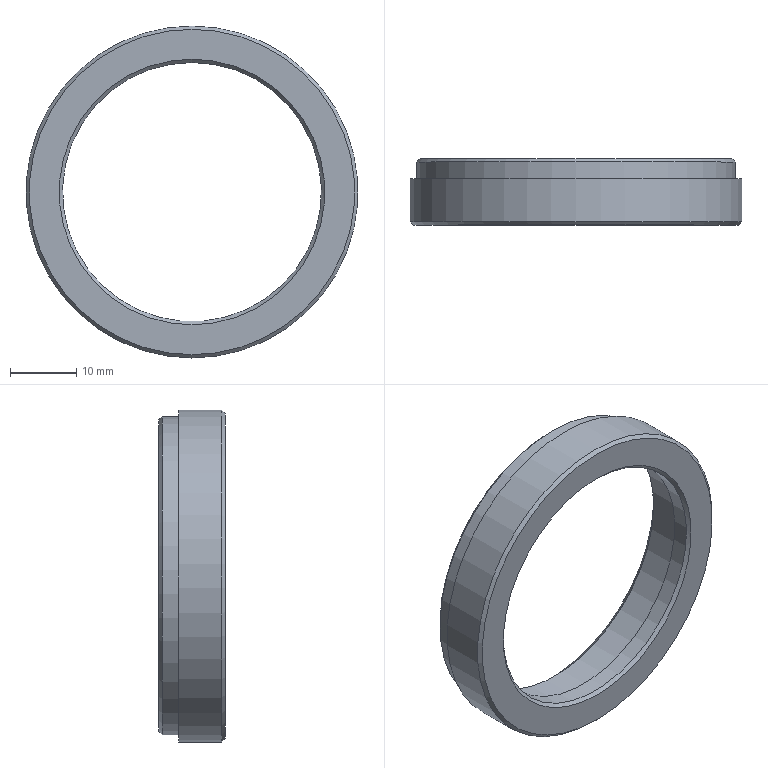Part | STEP file | JBJ-P-1018-01 | 1 solid | 12 faces | box 50 x 10 x 50 mm | volume 5771 mm3 | plane 4 | cylinder 4 | cone 4 | commonest cylinder face diameters 39 x1 42 x1 48 x1 50 x1
STEP:
#1=CARTESIAN_POINT('',(0.,10.,23.5));
#2=VERTEX_POINT('',#1);
#3=CARTESIAN_POINT('',(0.,10.,0.));
#4=DIRECTION('',(0.,1.,0.));
#5=DIRECTION('',(0.,0.,1.));
#6=AXIS2_PLACEMENT_3D('',#3,#4,#5);
#7=CIRCLE('',#6,23.5);
#8=EDGE_CURVE('',#2,#2,#7,.T.);
#9=ORIENTED_EDGE('',*,*,#8,.T.);
#10=EDGE_LOOP('',(#9));
#11=FACE_OUTER_BOUND('',#10,.T.);
#12=CARTESIAN_POINT('',(0.,10.,22.));
#13=VERTEX_POINT('',#12);
#14=CARTESIAN_POINT('',(0.,10.,0.));
#15=DIRECTION('',(0.,-1.,0.));
#16=DIRECTION('',(0.,0.,1.));
#17=AXIS2_PLACEMENT_3D('',#14,#15,#16);
#18=CIRCLE('',#17,22.);
#19=EDGE_CURVE('',#13,#13,#18,.T.);
#20=ORIENTED_EDGE('',*,*,#19,.T.);
#21=EDGE_LOOP('',(#20));
#22=FACE_BOUND('',#21,.T.);
#23=CARTESIAN_POINT('',(0.,10.,0.));
#24=DIRECTION('',(0.,1.,0.));
#25=DIRECTION('',(0.,0.,1.));
#26=AXIS2_PLACEMENT_3D('',#23,#24,#25);
#27=PLANE('',#26);
#28=ADVANCED_FACE('',(#11,#22),#27,.T.);
#29=CARTESIAN_POINT('',(0.,0.5,25.));
#30=VERTEX_POINT('',#29);
#31=CARTESIAN_POINT('',(0.,0.5,0.));
#32=DIRECTION('',(0.,1.,0.));
#33=DIRECTION('',(0.,0.,1.));
#34=AXIS2_PLACEMENT_3D('',#31,#32,#33);
#35=CIRCLE('',#34,25.);
#36=EDGE_CURVE('',#30,#30,#35,.T.);
#37=ORIENTED_EDGE('',*,*,#36,.T.);
#38=EDGE_LOOP('',(#37));
#39=FACE_OUTER_BOUND('',#38,.T.);
#40=CARTESIAN_POINT('',(0.,7.,25.));
#41=VERTEX_POINT('',#40);
#42=CARTESIAN_POINT('',(0.,7.,0.));
#43=DIRECTION('',(0.,1.,0.));
#44=DIRECTION('',(0.,0.,1.));
#45=AXIS2_PLACEMENT_3D('',#42,#43,#44);
#46=CIRCLE('',#45,25.);
#47=EDGE_CURVE('',#41,#41,#46,.T.);
#48=ORIENTED_EDGE('',*,*,#47,.F.);
#49=EDGE_LOOP('',(#48));
#50=FACE_OUTER_BOUND('',#49,.T.);
#51=CARTESIAN_POINT('',(0.,10.,0.));
#52=DIRECTION('',(0.,-1.,0.));
#53=DIRECTION('',(0.,0.,-1.));
#54=AXIS2_PLACEMENT_3D('',#51,#52,#53);
#55=CYLINDRICAL_SURFACE('',#54,25.);
#56=ADVANCED_FACE('',(#39,#50),#55,.T.);
#57=CARTESIAN_POINT('',(0.,0.5,19.5));
#58=VERTEX_POINT('',#57);
#59=CARTESIAN_POINT('',(0.,0.5,0.));
#60=DIRECTION('',(0.,-1.,0.));
#61=DIRECTION('',(0.,0.,1.));
#62=AXIS2_PLACEMENT_3D('',#59,#60,#61);
#63=CIRCLE('',#62,19.5);
#64=EDGE_CURVE('',#58,#58,#63,.T.);
#65=ORIENTED_EDGE('',*,*,#64,.T.);
#66=EDGE_LOOP('',(#65));
#67=FACE_OUTER_BOUND('',#66,.T.);
#68=CARTESIAN_POINT('',(0.,3.,19.5));
#69=VERTEX_POINT('',#68);
#70=CARTESIAN_POINT('',(0.,3.,0.));
#71=DIRECTION('',(0.,1.,0.));
#72=DIRECTION('',(0.,0.,1.));
#73=AXIS2_PLACEMENT_3D('',#70,#71,#72);
#74=CIRCLE('',#73,19.5);
#75=EDGE_CURVE('',#69,#69,#74,.T.);
#76=ORIENTED_EDGE('',*,*,#75,.T.);
#77=EDGE_LOOP('',(#76));
#78=FACE_OUTER_BOUND('',#77,.T.);
#79=CARTESIAN_POINT('',(0.,10.,0.));
#80=DIRECTION('',(0.,-1.,0.));
#81=DIRECTION('',(0.,0.,-1.));
#82=AXIS2_PLACEMENT_3D('',#79,#80,#81);
#83=CYLINDRICAL_SURFACE('',#82,19.5);
#84=ADVANCED_FACE('',(#67,#78),#83,.F.);
#85=CARTESIAN_POINT('',(0.,0.,20.));
#86=VERTEX_POINT('',#85);
#87=CARTESIAN_POINT('',(0.,0.,0.));
#88=DIRECTION('',(0.,1.,0.));
#89=DIRECTION('',(0.,0.,1.));
#90=AXIS2_PLACEMENT_3D('',#87,#88,#89);
#91=CIRCLE('',#90,20.);
#92=EDGE_CURVE('',#86,#86,#91,.T.);
#93=ORIENTED_EDGE('',*,*,#92,.T.);
#94=EDGE_LOOP('',(#93));
#95=FACE_BOUND('',#94,.T.);
#96=CARTESIAN_POINT('',(0.,0.,24.5));
#97=VERTEX_POINT('',#96);
#98=CARTESIAN_POINT('',(0.,0.,0.));
#99=DIRECTION('',(0.,-1.,0.));
#100=DIRECTION('',(0.,0.,1.));
#101=AXIS2_PLACEMENT_3D('',#98,#99,#100);
#102=CIRCLE('',#101,24.5);
#103=EDGE_CURVE('',#97,#97,#102,.T.);
#104=ORIENTED_EDGE('',*,*,#103,.T.);
#105=EDGE_LOOP('',(#104));
#106=FACE_OUTER_BOUND('',#105,.T.);
#107=CARTESIAN_POINT('',(0.,0.,0.));
#108=DIRECTION('',(0.,1.,0.));
#109=DIRECTION('',(0.,0.,1.));
#110=AXIS2_PLACEMENT_3D('',#107,#108,#109);
#111=PLANE('',#110);
#112=ADVANCED_FACE('',(#95,#106),#111,.F.);
#113=CARTESIAN_POINT('',(0.,9.,21.));
#114=VERTEX_POINT('',#113);
#115=CARTESIAN_POINT('',(0.,9.,0.));
#116=DIRECTION('',(0.,1.,0.));
#117=DIRECTION('',(0.,0.,1.));
#118=AXIS2_PLACEMENT_3D('',#115,#116,#117);
#119=CIRCLE('',#118,21.);
#120=EDGE_CURVE('',#114,#114,#119,.T.);
#121=ORIENTED_EDGE('',*,*,#120,.T.);
#122=EDGE_LOOP('',(#121));
#123=FACE_OUTER_BOUND('',#122,.T.);
#124=CARTESIAN_POINT('',(0.,3.,21.));
#125=VERTEX_POINT('',#124);
#126=CARTESIAN_POINT('',(0.,3.,0.));
#127=DIRECTION('',(0.,1.,0.));
#128=DIRECTION('',(0.,0.,1.));
#129=AXIS2_PLACEMENT_3D('',#126,#127,#128);
#130=CIRCLE('',#129,21.);
#131=EDGE_CURVE('',#125,#125,#130,.T.);
#132=ORIENTED_EDGE('',*,*,#131,.F.);
#133=EDGE_LOOP('',(#132));
#134=FACE_OUTER_BOUND('',#133,.T.);
#135=CARTESIAN_POINT('',(0.,3.,0.));
#136=DIRECTION('',(0.,1.,0.));
#137=DIRECTION('',(0.,0.,1.));
#138=AXIS2_PLACEMENT_3D('',#135,#136,#137);
#139=CYLINDRICAL_SURFACE('',#138,21.);
#140=ADVANCED_FACE('',(#123,#134),#139,.F.);
#141=ORIENTED_EDGE('',*,*,#75,.F.);
#142=EDGE_LOOP('',(#141));
#143=FACE_BOUND('',#142,.T.);
#144=ORIENTED_EDGE('',*,*,#131,.T.);
#145=EDGE_LOOP('',(#144));
#146=FACE_OUTER_BOUND('',#145,.T.);
#147=CARTESIAN_POINT('',(0.,3.,0.));
#148=DIRECTION('',(0.,1.,0.));
#149=DIRECTION('',(0.,0.,1.));
#150=AXIS2_PLACEMENT_3D('',#147,#148,#149);
#151=PLANE('',#150);
#152=ADVANCED_FACE('',(#143,#146),#151,.T.);
#153=ORIENTED_EDGE('',*,*,#19,.F.);
#154=EDGE_LOOP('',(#153));
#155=FACE_OUTER_BOUND('',#154,.T.);
#156=ORIENTED_EDGE('',*,*,#120,.F.);
#157=EDGE_LOOP('',(#156));
#158=FACE_BOUND('',#157,.T.);
#159=CARTESIAN_POINT('',(0.,9.,0.));
#160=DIRECTION('',(0.,1.,0.));
#161=DIRECTION('',(0.,0.,1.));
#162=AXIS2_PLACEMENT_3D('',#159,#160,#161);
#163=CONICAL_SURFACE('',#162,21.,0.7854);
#164=ADVANCED_FACE('',(#155,#158),#163,.F.);
#165=CARTESIAN_POINT('',(0.,7.,24.));
#166=VERTEX_POINT('',#165);
#167=CARTESIAN_POINT('',(0.,7.,0.));
#168=DIRECTION('',(0.,1.,0.));
#169=DIRECTION('',(0.,0.,1.));
#170=AXIS2_PLACEMENT_3D('',#167,#168,#169);
#171=CIRCLE('',#170,24.);
#172=EDGE_CURVE('',#166,#166,#171,.T.);
#173=ORIENTED_EDGE('',*,*,#172,.F.);
#174=EDGE_LOOP('',(#173));
#175=FACE_BOUND('',#174,.T.);
#176=ORIENTED_EDGE('',*,*,#47,.T.);
#177=EDGE_LOOP('',(#176));
#178=FACE_OUTER_BOUND('',#177,.T.);
#179=CARTESIAN_POINT('',(0.,7.,0.));
#180=DIRECTION('',(0.,1.,0.));
#181=DIRECTION('',(0.,0.,1.));
#182=AXIS2_PLACEMENT_3D('',#179,#180,#181);
#183=PLANE('',#182);
#184=ADVANCED_FACE('',(#175,#178),#183,.T.);
#185=CARTESIAN_POINT('',(0.,9.5,24.));
#186=VERTEX_POINT('',#185);
#187=CARTESIAN_POINT('',(0.,9.5,0.));
#188=DIRECTION('',(0.,-1.,0.));
#189=DIRECTION('',(0.,0.,1.));
#190=AXIS2_PLACEMENT_3D('',#187,#188,#189);
#191=CIRCLE('',#190,24.);
#192=EDGE_CURVE('',#186,#186,#191,.T.);
#193=ORIENTED_EDGE('',*,*,#192,.T.);
#194=EDGE_LOOP('',(#193));
#195=FACE_OUTER_BOUND('',#194,.T.);
#196=ORIENTED_EDGE('',*,*,#172,.T.);
#197=EDGE_LOOP('',(#196));
#198=FACE_OUTER_BOUND('',#197,.T.);
#199=CARTESIAN_POINT('',(0.,7.,0.));
#200=DIRECTION('',(0.,1.,0.));
#201=DIRECTION('',(0.,0.,1.));
#202=AXIS2_PLACEMENT_3D('',#199,#200,#201);
#203=CYLINDRICAL_SURFACE('',#202,24.);
#204=ADVANCED_FACE('',(#195,#198),#203,.T.);
#205=ORIENTED_EDGE('',*,*,#64,.F.);
#206=EDGE_LOOP('',(#205));
#207=FACE_BOUND('',#206,.T.);
#208=ORIENTED_EDGE('',*,*,#92,.F.);
#209=EDGE_LOOP('',(#208));
#210=FACE_OUTER_BOUND('',#209,.T.);
#211=CARTESIAN_POINT('',(0.,0.,0.));
#212=DIRECTION('',(0.,-1.,0.));
#213=DIRECTION('',(0.,0.,-1.));
#214=AXIS2_PLACEMENT_3D('',#211,#212,#213);
#215=CONICAL_SURFACE('',#214,20.,0.7854);
#216=ADVANCED_FACE('',(#207,#210),#215,.F.);
#217=ORIENTED_EDGE('',*,*,#103,.F.);
#218=EDGE_LOOP('',(#217));
#219=FACE_BOUND('',#218,.T.);
#220=ORIENTED_EDGE('',*,*,#36,.F.);
#221=EDGE_LOOP('',(#220));
#222=FACE_OUTER_BOUND('',#221,.T.);
#223=CARTESIAN_POINT('',(0.,0.5,0.));
#224=DIRECTION('',(0.,1.,0.));
#225=DIRECTION('',(0.,0.,1.));
#226=AXIS2_PLACEMENT_3D('',#223,#224,#225);
#227=CONICAL_SURFACE('',#226,25.,0.7854);
#228=ADVANCED_FACE('',(#219,#222),#227,.T.);
#229=ORIENTED_EDGE('',*,*,#192,.F.);
#230=EDGE_LOOP('',(#229));
#231=FACE_OUTER_BOUND('',#230,.T.);
#232=ORIENTED_EDGE('',*,*,#8,.F.);
#233=EDGE_LOOP('',(#232));
#234=FACE_BOUND('',#233,.T.);
#235=CARTESIAN_POINT('',(0.,10.,0.));
#236=DIRECTION('',(0.,-1.,0.));
#237=DIRECTION('',(0.,0.,-1.));
#238=AXIS2_PLACEMENT_3D('',#235,#236,#237);
#239=CONICAL_SURFACE('',#238,23.5,0.7854);
#240=ADVANCED_FACE('',(#231,#234),#239,.T.);
#241=CLOSED_SHELL('',(#28,#56,#84,#112,#140,#152,#164,#184,#204,#216,#228,#240));
#242=MANIFOLD_SOLID_BREP('',#241);
#243=CARTESIAN_POINT('',(0.,0.,0.));
#244=DIRECTION('',(0.,0.,1.));
#245=DIRECTION('',(1.,0.,0.));
#246=AXIS2_PLACEMENT_3D('',#243,#244,#245);
#247=(LENGTH_UNIT()NAMED_UNIT(*)SI_UNIT(.MILLI.,.METRE.));
#248=UNCERTAINTY_MEASURE_WITH_UNIT(LENGTH_MEASURE(0.00001),#247,'','');
#249=(NAMED_UNIT(*)PLANE_ANGLE_UNIT()SI_UNIT($,.RADIAN.));
#250=(NAMED_UNIT(*)SI_UNIT($,.STERADIAN.)SOLID_ANGLE_UNIT());
#251=(GEOMETRIC_REPRESENTATION_CONTEXT(3)GLOBAL_UNCERTAINTY_ASSIGNED_CONTEXT((#248))GLOBAL_UNIT_ASSIGNED_CONTEXT((#247,#249,#250))REPRESENTATION_CONTEXT('',''));
#252=ADVANCED_BREP_SHAPE_REPRESENTATION('',(#242,#246),#251);